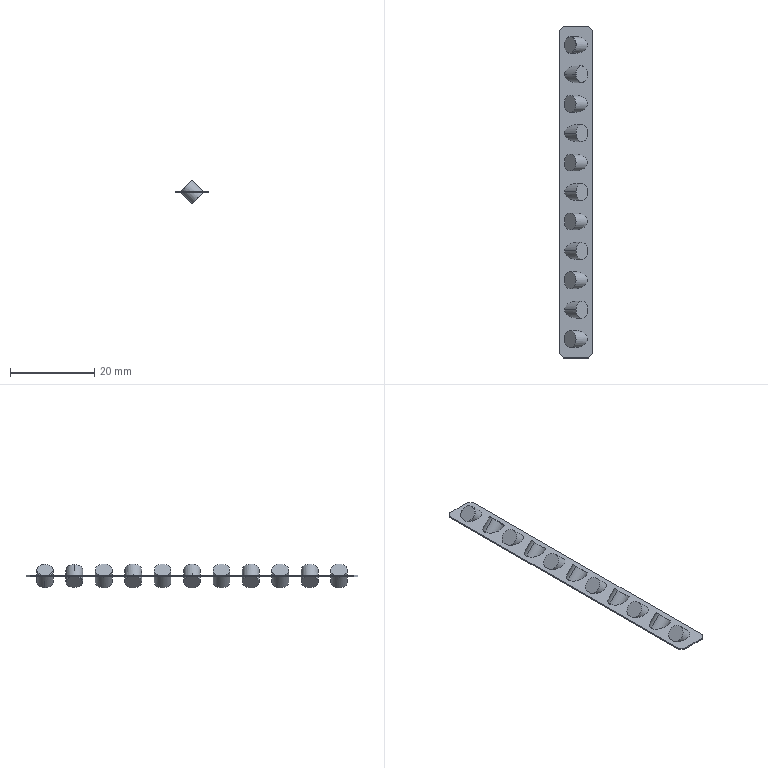Part | STEP file | 1 solid | 71 faces | box 8 x 79 x 5.657 mm | volume 683.542 mm3 | cylinder 33 | plane 32 | cone 6 | commonest cylinder face diameters 4 x33